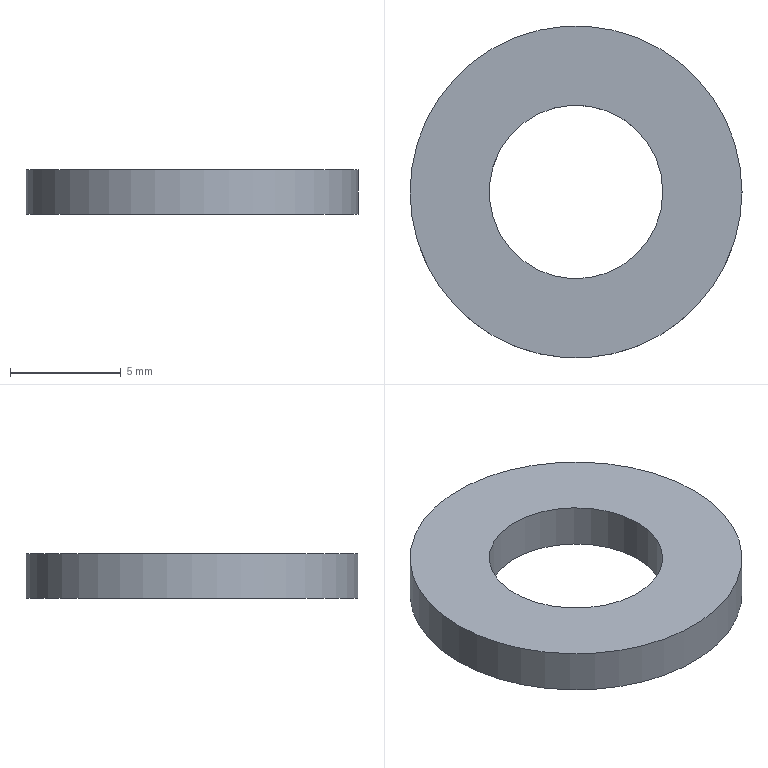Part | NX | features DATUM_CSYS 2, EXTRUDE 1, OFFSET_REGION 1, SKETCH 1 | 1 solid | 4 faces | box 15 x 15 x 2 mm | volume 256.846 mm3 | cylinder 2 | plane 2 | commonest cylinder face diameters 7.841 x1 15 x1
STEP:
#1=CARTESIAN_POINT('',(7.5,0.,2.));
#2=VERTEX_POINT('',#1);
#3=CARTESIAN_POINT('',(0.,0.,2.));
#4=DIRECTION('',(0.,0.,1.));
#5=DIRECTION('',(1.,0.,0.));
#6=AXIS2_PLACEMENT_3D('',#3,#4,#5);
#7=CIRCLE('',#6,7.5);
#8=EDGE_CURVE('',#2,#2,#7,.T.);
#9=ORIENTED_EDGE('',*,*,#8,.F.);
#10=EDGE_LOOP('',(#9));
#11=FACE_BOUND('',#10,.T.);
#12=CARTESIAN_POINT('',(7.5,0.,0.));
#13=VERTEX_POINT('',#12);
#14=CARTESIAN_POINT('',(0.,0.,0.));
#15=DIRECTION('',(0.,0.,1.));
#16=DIRECTION('',(1.,0.,0.));
#17=AXIS2_PLACEMENT_3D('',#14,#15,#16);
#18=CIRCLE('',#17,7.5);
#19=EDGE_CURVE('',#13,#13,#18,.T.);
#20=ORIENTED_EDGE('',*,*,#19,.T.);
#21=EDGE_LOOP('',(#20));
#22=FACE_BOUND('',#21,.T.);
#23=CARTESIAN_POINT('',(0.,0.,2.));
#24=DIRECTION('',(0.,0.,-1.));
#25=DIRECTION('',(-1.,0.,0.));
#26=AXIS2_PLACEMENT_3D('',#23,#24,#25);
#27=CYLINDRICAL_SURFACE('',#26,7.5);
#28=ADVANCED_FACE('',(#11,#22),#27,.T.);
#29=CARTESIAN_POINT('',(3.921,0.,2.));
#30=VERTEX_POINT('',#29);
#31=CARTESIAN_POINT('',(0.,0.,2.));
#32=DIRECTION('',(0.,0.,1.));
#33=DIRECTION('',(1.,0.,0.));
#34=AXIS2_PLACEMENT_3D('',#31,#32,#33);
#35=CIRCLE('',#34,3.921);
#36=EDGE_CURVE('',#30,#30,#35,.T.);
#37=ORIENTED_EDGE('',*,*,#36,.T.);
#38=EDGE_LOOP('',(#37));
#39=FACE_BOUND('',#38,.T.);
#40=CARTESIAN_POINT('',(3.921,0.,0.));
#41=VERTEX_POINT('',#40);
#42=CARTESIAN_POINT('',(0.,0.,0.));
#43=DIRECTION('',(0.,0.,1.));
#44=DIRECTION('',(1.,0.,0.));
#45=AXIS2_PLACEMENT_3D('',#42,#43,#44);
#46=CIRCLE('',#45,3.921);
#47=EDGE_CURVE('',#41,#41,#46,.T.);
#48=ORIENTED_EDGE('',*,*,#47,.F.);
#49=EDGE_LOOP('',(#48));
#50=FACE_BOUND('',#49,.T.);
#51=CARTESIAN_POINT('',(0.,0.,2.));
#52=DIRECTION('',(0.,0.,-1.));
#53=DIRECTION('',(-1.,0.,0.));
#54=AXIS2_PLACEMENT_3D('',#51,#52,#53);
#55=CYLINDRICAL_SURFACE('',#54,3.921);
#56=ADVANCED_FACE('',(#39,#50),#55,.F.);
#57=ORIENTED_EDGE('',*,*,#8,.T.);
#58=EDGE_LOOP('',(#57));
#59=FACE_BOUND('',#58,.T.);
#60=ORIENTED_EDGE('',*,*,#36,.F.);
#61=EDGE_LOOP('',(#60));
#62=FACE_BOUND('',#61,.T.);
#63=CARTESIAN_POINT('',(0.,0.,2.));
#64=DIRECTION('',(0.,0.,1.));
#65=DIRECTION('',(1.,0.,0.));
#66=AXIS2_PLACEMENT_3D('',#63,#64,#65);
#67=PLANE('',#66);
#68=ADVANCED_FACE('',(#59,#62),#67,.T.);
#69=ORIENTED_EDGE('',*,*,#19,.F.);
#70=EDGE_LOOP('',(#69));
#71=FACE_BOUND('',#70,.T.);
#72=ORIENTED_EDGE('',*,*,#47,.T.);
#73=EDGE_LOOP('',(#72));
#74=FACE_BOUND('',#73,.T.);
#75=CARTESIAN_POINT('',(0.,0.,0.));
#76=DIRECTION('',(0.,0.,1.));
#77=DIRECTION('',(1.,0.,0.));
#78=AXIS2_PLACEMENT_3D('',#75,#76,#77);
#79=PLANE('',#78);
#80=ADVANCED_FACE('',(#71,#74),#79,.F.);
#81=CLOSED_SHELL('',(#28,#56,#68,#80));
#82=MANIFOLD_SOLID_BREP('',#81);
#83=(LENGTH_UNIT()NAMED_UNIT(*)SI_UNIT(.MILLI.,.METRE.));
#84=UNCERTAINTY_MEASURE_WITH_UNIT(LENGTH_MEASURE(0.00001),#83,'','');
#85=(NAMED_UNIT(*)PLANE_ANGLE_UNIT()SI_UNIT($,.RADIAN.));
#86=(NAMED_UNIT(*)SI_UNIT($,.STERADIAN.)SOLID_ANGLE_UNIT());
#87=(GEOMETRIC_REPRESENTATION_CONTEXT(3)GLOBAL_UNCERTAINTY_ASSIGNED_CONTEXT((#84))GLOBAL_UNIT_ASSIGNED_CONTEXT((#83,#85,#86))REPRESENTATION_CONTEXT('',''));
#88=ADVANCED_BREP_SHAPE_REPRESENTATION('',(#82),#87);